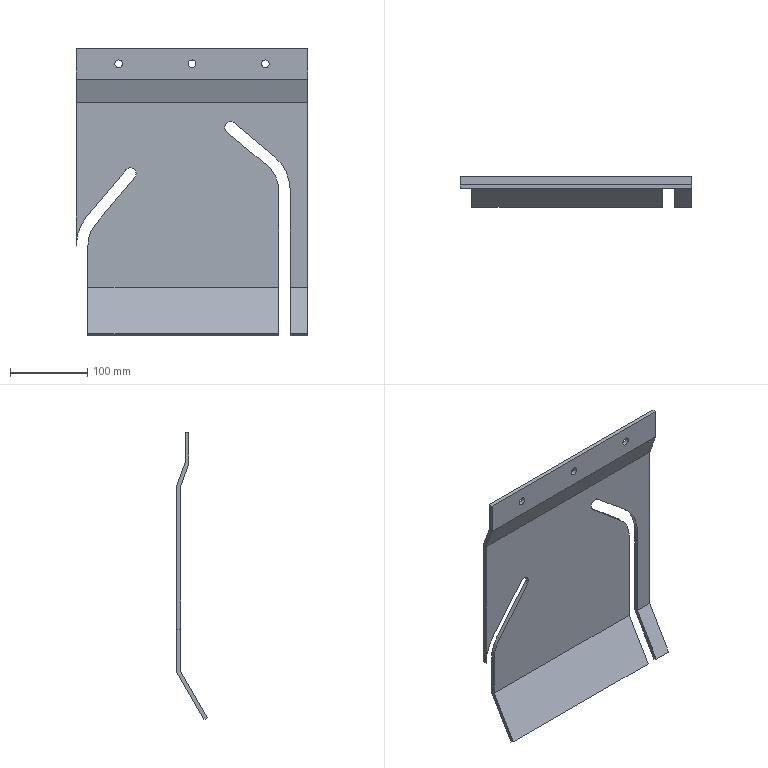Part | STEP file | gudingzhezhiban1 | 1 solid | 31 faces | box 300 x 39.641 x 372.5 mm | volume 530723 mm3 | plane 22 | cylinder 9 | commonest cylinder face diameters 10 x3 15 x2 85 x2 115 x2